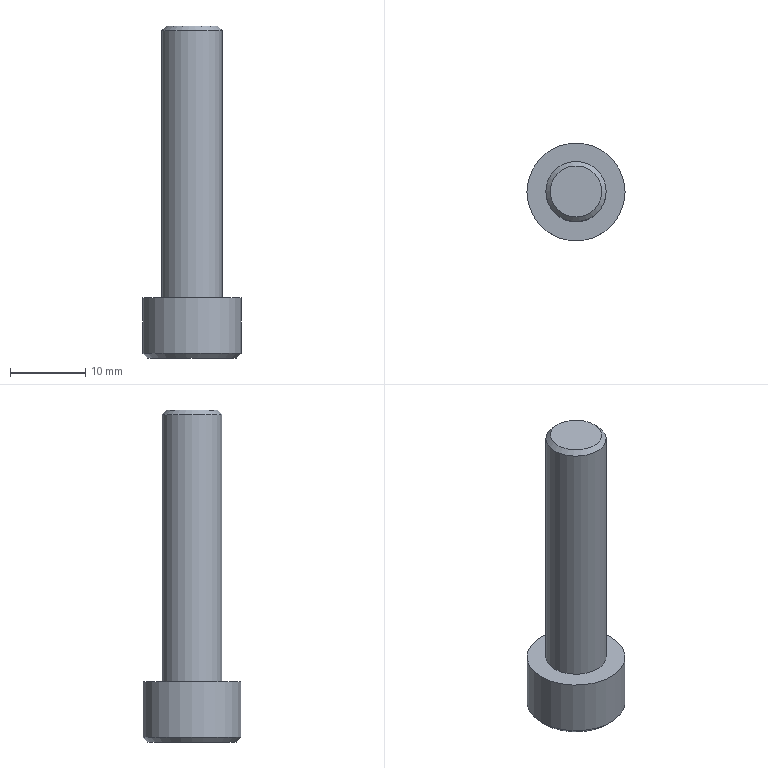Part | NX | features M8.00-35.00 2 | 1 solid | 14 faces | box 13 x 13 x 44 mm | volume 2700 mm3 | plane 10 | cylinder 2 | cone 2 | commonest cylinder face diameters 8 x1 13 x1
STEP:
#1=CARTESIAN_POINT('',(-60.9,-50.,-269.5));
#2=VERTEX_POINT('',#1);
#3=CARTESIAN_POINT('',(-55.,-50.,-269.5));
#4=DIRECTION('',(0.,0.,-1.));
#5=DIRECTION('',(-1.,0.,0.));
#6=AXIS2_PLACEMENT_3D('',#3,#4,#5);
#7=CIRCLE('',#6,5.9);
#8=EDGE_CURVE('',#2,#2,#7,.T.);
#9=ORIENTED_EDGE('',*,*,#8,.T.);
#10=EDGE_LOOP('',(#9));
#11=FACE_BOUND('',#10,.T.);
#12=CARTESIAN_POINT('',(-51.6,-48.037,-269.5));
#13=VERTEX_POINT('',#12);
#14=CARTESIAN_POINT('',(-51.6,-51.963,-269.5));
#15=VERTEX_POINT('',#14);
#16=CARTESIAN_POINT('',(-51.6,-48.037,-269.5));
#17=DIRECTION('',(0.,-1.,0.));
#18=VECTOR('',#17,1000.);
#19=LINE('',#16,#18);
#20=EDGE_CURVE('',#13,#15,#19,.T.);
#21=ORIENTED_EDGE('',*,*,#20,.F.);
#22=CARTESIAN_POINT('',(-55.,-46.074,-269.5));
#23=VERTEX_POINT('',#22);
#24=CARTESIAN_POINT('',(-55.,-46.074,-269.5));
#25=DIRECTION('',(0.866,-0.5,0.));
#26=VECTOR('',#25,1000.);
#27=LINE('',#24,#26);
#28=EDGE_CURVE('',#23,#13,#27,.T.);
#29=ORIENTED_EDGE('',*,*,#28,.F.);
#30=CARTESIAN_POINT('',(-58.4,-48.037,-269.5));
#31=VERTEX_POINT('',#30);
#32=CARTESIAN_POINT('',(-58.4,-48.037,-269.5));
#33=DIRECTION('',(0.866,0.5,0.));
#34=VECTOR('',#33,1000.);
#35=LINE('',#32,#34);
#36=EDGE_CURVE('',#31,#23,#35,.T.);
#37=ORIENTED_EDGE('',*,*,#36,.F.);
#38=CARTESIAN_POINT('',(-58.4,-51.963,-269.5));
#39=VERTEX_POINT('',#38);
#40=CARTESIAN_POINT('',(-58.4,-51.963,-269.5));
#41=DIRECTION('',(0.,1.,0.));
#42=VECTOR('',#41,1000.);
#43=LINE('',#40,#42);
#44=EDGE_CURVE('',#39,#31,#43,.T.);
#45=ORIENTED_EDGE('',*,*,#44,.F.);
#46=CARTESIAN_POINT('',(-55.,-53.926,-269.5));
#47=VERTEX_POINT('',#46);
#48=CARTESIAN_POINT('',(-55.,-53.926,-269.5));
#49=DIRECTION('',(-0.866,0.5,0.));
#50=VECTOR('',#49,1000.);
#51=LINE('',#48,#50);
#52=EDGE_CURVE('',#47,#39,#51,.T.);
#53=ORIENTED_EDGE('',*,*,#52,.F.);
#54=CARTESIAN_POINT('',(-51.6,-51.963,-269.5));
#55=DIRECTION('',(-0.866,-0.5,0.));
#56=VECTOR('',#55,1000.);
#57=LINE('',#54,#56);
#58=EDGE_CURVE('',#15,#47,#57,.T.);
#59=ORIENTED_EDGE('',*,*,#58,.F.);
#60=EDGE_LOOP('',(#21,#29,#37,#45,#53,#59));
#61=FACE_BOUND('',#60,.T.);
#62=CARTESIAN_POINT('',(-55.,-50.,-269.5));
#63=DIRECTION('',(0.,0.,-1.));
#64=DIRECTION('',(-1.,0.,0.));
#65=AXIS2_PLACEMENT_3D('',#62,#63,#64);
#66=PLANE('',#65);
#67=ADVANCED_FACE('',(#11,#61),#66,.T.);
#68=CARTESIAN_POINT('',(-51.,-50.,-261.5));
#69=VERTEX_POINT('',#68);
#70=CARTESIAN_POINT('',(-55.,-50.,-261.5));
#71=DIRECTION('',(0.,0.,1.));
#72=DIRECTION('',(1.,0.,0.));
#73=AXIS2_PLACEMENT_3D('',#70,#71,#72);
#74=CIRCLE('',#73,4.);
#75=EDGE_CURVE('',#69,#69,#74,.T.);
#76=ORIENTED_EDGE('',*,*,#75,.F.);
#77=EDGE_LOOP('',(#76));
#78=FACE_BOUND('',#77,.T.);
#79=CARTESIAN_POINT('',(-48.5,-50.,-261.5));
#80=VERTEX_POINT('',#79);
#81=CARTESIAN_POINT('',(-55.,-50.,-261.5));
#82=DIRECTION('',(0.,0.,-1.));
#83=DIRECTION('',(1.,0.,0.));
#84=AXIS2_PLACEMENT_3D('',#81,#82,#83);
#85=CIRCLE('',#84,6.5);
#86=EDGE_CURVE('',#80,#80,#85,.T.);
#87=ORIENTED_EDGE('',*,*,#86,.F.);
#88=EDGE_LOOP('',(#87));
#89=FACE_BOUND('',#88,.T.);
#90=CARTESIAN_POINT('',(-55.,-50.,-261.5));
#91=DIRECTION('',(0.,0.,1.));
#92=DIRECTION('',(1.,0.,0.));
#93=AXIS2_PLACEMENT_3D('',#90,#91,#92);
#94=PLANE('',#93);
#95=ADVANCED_FACE('',(#78,#89),#94,.T.);
#96=CARTESIAN_POINT('',(-61.5,-50.,-268.9));
#97=VERTEX_POINT('',#96);
#98=CARTESIAN_POINT('',(-55.,-50.,-268.9));
#99=DIRECTION('',(0.,0.,-1.));
#100=DIRECTION('',(-1.,0.,0.));
#101=AXIS2_PLACEMENT_3D('',#98,#99,#100);
#102=CIRCLE('',#101,6.5);
#103=EDGE_CURVE('',#97,#97,#102,.F.);
#104=ORIENTED_EDGE('',*,*,#103,.T.);
#105=EDGE_LOOP('',(#104));
#106=FACE_BOUND('',#105,.T.);
#107=ORIENTED_EDGE('',*,*,#86,.T.);
#108=EDGE_LOOP('',(#107));
#109=FACE_BOUND('',#108,.T.);
#110=CARTESIAN_POINT('',(-55.,-50.,-261.5));
#111=DIRECTION('',(0.,0.,-1.));
#112=DIRECTION('',(1.,0.,0.));
#113=AXIS2_PLACEMENT_3D('',#110,#111,#112);
#114=CYLINDRICAL_SURFACE('',#113,6.5);
#115=ADVANCED_FACE('',(#106,#109),#114,.T.);
#116=CARTESIAN_POINT('',(-51.6,-50.,-225.5));
#117=VERTEX_POINT('',#116);
#118=CARTESIAN_POINT('',(-55.,-50.,-225.5));
#119=DIRECTION('',(0.,0.,1.));
#120=DIRECTION('',(1.,0.,0.));
#121=AXIS2_PLACEMENT_3D('',#118,#119,#120);
#122=CIRCLE('',#121,3.4);
#123=EDGE_CURVE('',#117,#117,#122,.T.);
#124=ORIENTED_EDGE('',*,*,#123,.T.);
#125=EDGE_LOOP('',(#124));
#126=FACE_BOUND('',#125,.T.);
#127=CARTESIAN_POINT('',(-55.,-50.,-225.5));
#128=DIRECTION('',(0.,0.,1.));
#129=DIRECTION('',(1.,0.,0.));
#130=AXIS2_PLACEMENT_3D('',#127,#128,#129);
#131=PLANE('',#130);
#132=ADVANCED_FACE('',(#126),#131,.T.);
#133=CARTESIAN_POINT('',(-51.,-50.,-226.1));
#134=VERTEX_POINT('',#133);
#135=CARTESIAN_POINT('',(-55.,-50.,-226.1));
#136=DIRECTION('',(0.,0.,1.));
#137=DIRECTION('',(1.,0.,0.));
#138=AXIS2_PLACEMENT_3D('',#135,#136,#137);
#139=CIRCLE('',#138,4.);
#140=EDGE_CURVE('',#134,#134,#139,.F.);
#141=ORIENTED_EDGE('',*,*,#140,.T.);
#142=EDGE_LOOP('',(#141));
#143=FACE_BOUND('',#142,.T.);
#144=ORIENTED_EDGE('',*,*,#75,.T.);
#145=EDGE_LOOP('',(#144));
#146=FACE_BOUND('',#145,.T.);
#147=CARTESIAN_POINT('',(-55.,-50.,-261.5));
#148=DIRECTION('',(0.,0.,1.));
#149=DIRECTION('',(1.,0.,0.));
#150=AXIS2_PLACEMENT_3D('',#147,#148,#149);
#151=CYLINDRICAL_SURFACE('',#150,4.);
#152=ADVANCED_FACE('',(#143,#146),#151,.T.);
#153=ORIENTED_EDGE('',*,*,#58,.T.);
#154=CARTESIAN_POINT('',(-55.,-53.926,-265.5));
#155=VERTEX_POINT('',#154);
#156=CARTESIAN_POINT('',(-55.,-53.926,-265.5));
#157=DIRECTION('',(0.,0.,-1.));
#158=VECTOR('',#157,1000.);
#159=LINE('',#156,#158);
#160=EDGE_CURVE('',#47,#155,#159,.F.);
#161=ORIENTED_EDGE('',*,*,#160,.T.);
#162=CARTESIAN_POINT('',(-51.6,-51.963,-265.5));
#163=VERTEX_POINT('',#162);
#164=CARTESIAN_POINT('',(-51.6,-51.963,-265.5));
#165=DIRECTION('',(-0.866,-0.5,0.));
#166=VECTOR('',#165,1000.);
#167=LINE('',#164,#166);
#168=EDGE_CURVE('',#155,#163,#167,.F.);
#169=ORIENTED_EDGE('',*,*,#168,.T.);
#170=CARTESIAN_POINT('',(-51.6,-51.963,-265.5));
#171=DIRECTION('',(0.,0.,-1.));
#172=VECTOR('',#171,1000.);
#173=LINE('',#170,#172);
#174=EDGE_CURVE('',#15,#163,#173,.F.);
#175=ORIENTED_EDGE('',*,*,#174,.F.);
#176=EDGE_LOOP('',(#153,#161,#169,#175));
#177=FACE_BOUND('',#176,.T.);
#178=CARTESIAN_POINT('',(-53.3,-52.944,-267.5));
#179=DIRECTION('',(0.5,-0.866,0.));
#180=DIRECTION('',(0.866,0.5,0.));
#181=AXIS2_PLACEMENT_3D('',#178,#179,#180);
#182=PLANE('',#181);
#183=ADVANCED_FACE('',(#177),#182,.F.);
#184=ORIENTED_EDGE('',*,*,#20,.T.);
#185=ORIENTED_EDGE('',*,*,#174,.T.);
#186=CARTESIAN_POINT('',(-51.6,-48.037,-265.5));
#187=VERTEX_POINT('',#186);
#188=CARTESIAN_POINT('',(-51.6,-48.037,-265.5));
#189=DIRECTION('',(0.,-1.,0.));
#190=VECTOR('',#189,1000.);
#191=LINE('',#188,#190);
#192=EDGE_CURVE('',#163,#187,#191,.F.);
#193=ORIENTED_EDGE('',*,*,#192,.T.);
#194=CARTESIAN_POINT('',(-51.6,-48.037,-265.5));
#195=DIRECTION('',(0.,0.,-1.));
#196=VECTOR('',#195,1000.);
#197=LINE('',#194,#196);
#198=EDGE_CURVE('',#13,#187,#197,.F.);
#199=ORIENTED_EDGE('',*,*,#198,.F.);
#200=EDGE_LOOP('',(#184,#185,#193,#199));
#201=FACE_BOUND('',#200,.T.);
#202=CARTESIAN_POINT('',(-51.6,-50.,-267.5));
#203=DIRECTION('',(1.,0.,0.));
#204=DIRECTION('',(0.,0.,-1.));
#205=AXIS2_PLACEMENT_3D('',#202,#203,#204);
#206=PLANE('',#205);
#207=ADVANCED_FACE('',(#201),#206,.F.);
#208=ORIENTED_EDGE('',*,*,#28,.T.);
#209=ORIENTED_EDGE('',*,*,#198,.T.);
#210=CARTESIAN_POINT('',(-55.,-46.074,-265.5));
#211=VERTEX_POINT('',#210);
#212=CARTESIAN_POINT('',(-55.,-46.074,-265.5));
#213=DIRECTION('',(0.866,-0.5,0.));
#214=VECTOR('',#213,1000.);
#215=LINE('',#212,#214);
#216=EDGE_CURVE('',#187,#211,#215,.F.);
#217=ORIENTED_EDGE('',*,*,#216,.T.);
#218=CARTESIAN_POINT('',(-55.,-46.074,-265.5));
#219=DIRECTION('',(0.,0.,-1.));
#220=VECTOR('',#219,1000.);
#221=LINE('',#218,#220);
#222=EDGE_CURVE('',#23,#211,#221,.F.);
#223=ORIENTED_EDGE('',*,*,#222,.F.);
#224=EDGE_LOOP('',(#208,#209,#217,#223));
#225=FACE_BOUND('',#224,.T.);
#226=CARTESIAN_POINT('',(-53.3,-47.056,-267.5));
#227=DIRECTION('',(0.5,0.866,0.));
#228=DIRECTION('',(-0.866,0.5,0.));
#229=AXIS2_PLACEMENT_3D('',#226,#227,#228);
#230=PLANE('',#229);
#231=ADVANCED_FACE('',(#225),#230,.F.);
#232=ORIENTED_EDGE('',*,*,#36,.T.);
#233=ORIENTED_EDGE('',*,*,#222,.T.);
#234=CARTESIAN_POINT('',(-58.4,-48.037,-265.5));
#235=VERTEX_POINT('',#234);
#236=CARTESIAN_POINT('',(-58.4,-48.037,-265.5));
#237=DIRECTION('',(0.866,0.5,0.));
#238=VECTOR('',#237,1000.);
#239=LINE('',#236,#238);
#240=EDGE_CURVE('',#211,#235,#239,.F.);
#241=ORIENTED_EDGE('',*,*,#240,.T.);
#242=CARTESIAN_POINT('',(-58.4,-48.037,-265.5));
#243=DIRECTION('',(0.,0.,-1.));
#244=VECTOR('',#243,1000.);
#245=LINE('',#242,#244);
#246=EDGE_CURVE('',#31,#235,#245,.F.);
#247=ORIENTED_EDGE('',*,*,#246,.F.);
#248=EDGE_LOOP('',(#232,#233,#241,#247));
#249=FACE_BOUND('',#248,.T.);
#250=CARTESIAN_POINT('',(-56.7,-47.056,-267.5));
#251=DIRECTION('',(-0.5,0.866,0.));
#252=DIRECTION('',(-0.866,-0.5,0.));
#253=AXIS2_PLACEMENT_3D('',#250,#251,#252);
#254=PLANE('',#253);
#255=ADVANCED_FACE('',(#249),#254,.F.);
#256=ORIENTED_EDGE('',*,*,#44,.T.);
#257=ORIENTED_EDGE('',*,*,#246,.T.);
#258=CARTESIAN_POINT('',(-58.4,-51.963,-265.5));
#259=VERTEX_POINT('',#258);
#260=CARTESIAN_POINT('',(-58.4,-51.963,-265.5));
#261=DIRECTION('',(0.,1.,0.));
#262=VECTOR('',#261,1000.);
#263=LINE('',#260,#262);
#264=EDGE_CURVE('',#235,#259,#263,.F.);
#265=ORIENTED_EDGE('',*,*,#264,.T.);
#266=CARTESIAN_POINT('',(-58.4,-51.963,-265.5));
#267=DIRECTION('',(0.,0.,-1.));
#268=VECTOR('',#267,1000.);
#269=LINE('',#266,#268);
#270=EDGE_CURVE('',#39,#259,#269,.F.);
#271=ORIENTED_EDGE('',*,*,#270,.F.);
#272=EDGE_LOOP('',(#256,#257,#265,#271));
#273=FACE_BOUND('',#272,.T.);
#274=CARTESIAN_POINT('',(-58.4,-50.,-267.5));
#275=DIRECTION('',(-1.,0.,0.));
#276=DIRECTION('',(0.,0.,1.));
#277=AXIS2_PLACEMENT_3D('',#274,#275,#276);
#278=PLANE('',#277);
#279=ADVANCED_FACE('',(#273),#278,.F.);
#280=ORIENTED_EDGE('',*,*,#52,.T.);
#281=ORIENTED_EDGE('',*,*,#270,.T.);
#282=CARTESIAN_POINT('',(-55.,-53.926,-265.5));
#283=DIRECTION('',(-0.866,0.5,0.));
#284=VECTOR('',#283,1000.);
#285=LINE('',#282,#284);
#286=EDGE_CURVE('',#259,#155,#285,.F.);
#287=ORIENTED_EDGE('',*,*,#286,.T.);
#288=ORIENTED_EDGE('',*,*,#160,.F.);
#289=EDGE_LOOP('',(#280,#281,#287,#288));
#290=FACE_BOUND('',#289,.T.);
#291=CARTESIAN_POINT('',(-56.7,-52.944,-267.5));
#292=DIRECTION('',(-0.5,-0.866,0.));
#293=DIRECTION('',(0.866,-0.5,0.));
#294=AXIS2_PLACEMENT_3D('',#291,#292,#293);
#295=PLANE('',#294);
#296=ADVANCED_FACE('',(#290),#295,.F.);
#297=ORIENTED_EDGE('',*,*,#286,.F.);
#298=ORIENTED_EDGE('',*,*,#264,.F.);
#299=ORIENTED_EDGE('',*,*,#240,.F.);
#300=ORIENTED_EDGE('',*,*,#216,.F.);
#301=ORIENTED_EDGE('',*,*,#192,.F.);
#302=ORIENTED_EDGE('',*,*,#168,.F.);
#303=EDGE_LOOP('',(#297,#298,#299,#300,#301,#302));
#304=FACE_BOUND('',#303,.T.);
#305=CARTESIAN_POINT('',(-55.,-50.,-265.5));
#306=DIRECTION('',(0.,0.,1.));
#307=DIRECTION('',(1.,0.,0.));
#308=AXIS2_PLACEMENT_3D('',#305,#306,#307);
#309=PLANE('',#308);
#310=ADVANCED_FACE('',(#304),#309,.F.);
#311=ORIENTED_EDGE('',*,*,#123,.F.);
#312=EDGE_LOOP('',(#311));
#313=FACE_BOUND('',#312,.T.);
#314=ORIENTED_EDGE('',*,*,#140,.F.);
#315=EDGE_LOOP('',(#314));
#316=FACE_BOUND('',#315,.T.);
#317=CARTESIAN_POINT('',(-55.,-50.,-226.1));
#318=DIRECTION('',(0.,0.,-1.));
#319=DIRECTION('',(-1.,0.,0.));
#320=AXIS2_PLACEMENT_3D('',#317,#318,#319);
#321=CONICAL_SURFACE('',#320,4.,0.7854);
#322=ADVANCED_FACE('',(#313,#316),#321,.T.);
#323=ORIENTED_EDGE('',*,*,#8,.F.);
#324=EDGE_LOOP('',(#323));
#325=FACE_BOUND('',#324,.T.);
#326=ORIENTED_EDGE('',*,*,#103,.F.);
#327=EDGE_LOOP('',(#326));
#328=FACE_BOUND('',#327,.T.);
#329=CARTESIAN_POINT('',(-55.,-50.,-268.9));
#330=DIRECTION('',(0.,0.,1.));
#331=DIRECTION('',(1.,0.,0.));
#332=AXIS2_PLACEMENT_3D('',#329,#330,#331);
#333=CONICAL_SURFACE('',#332,6.5,0.7854);
#334=ADVANCED_FACE('',(#325,#328),#333,.T.);
#335=CLOSED_SHELL('',(#67,#95,#115,#132,#152,#183,#207,#231,#255,#279,#296,#310,#322,#334));
#336=MANIFOLD_SOLID_BREP('',#335);
#337=(LENGTH_UNIT()NAMED_UNIT(*)SI_UNIT(.MILLI.,.METRE.));
#338=UNCERTAINTY_MEASURE_WITH_UNIT(LENGTH_MEASURE(0.00001),#337,'','');
#339=(NAMED_UNIT(*)PLANE_ANGLE_UNIT()SI_UNIT($,.RADIAN.));
#340=(NAMED_UNIT(*)SI_UNIT($,.STERADIAN.)SOLID_ANGLE_UNIT());
#341=(GEOMETRIC_REPRESENTATION_CONTEXT(3)GLOBAL_UNCERTAINTY_ASSIGNED_CONTEXT((#338))GLOBAL_UNIT_ASSIGNED_CONTEXT((#337,#339,#340))REPRESENTATION_CONTEXT('',''));
#342=ADVANCED_BREP_SHAPE_REPRESENTATION('',(#336),#341);